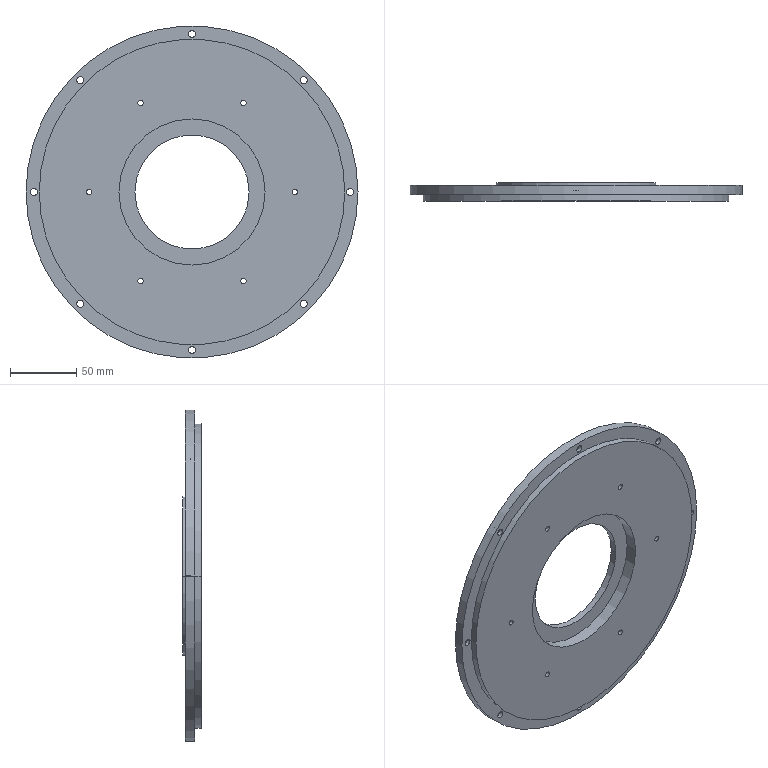Part | SolidWorks | features Cut 3, Revolution 1 | 1 solid | 70 faces | box 250 x 14 x 250 mm | volume 269051 mm3 | cylinder 56 | plane 14 | commonest cylinder face diameters 5.3 x16 10 x16 4 x12 86 x2 110 x2 120 x2